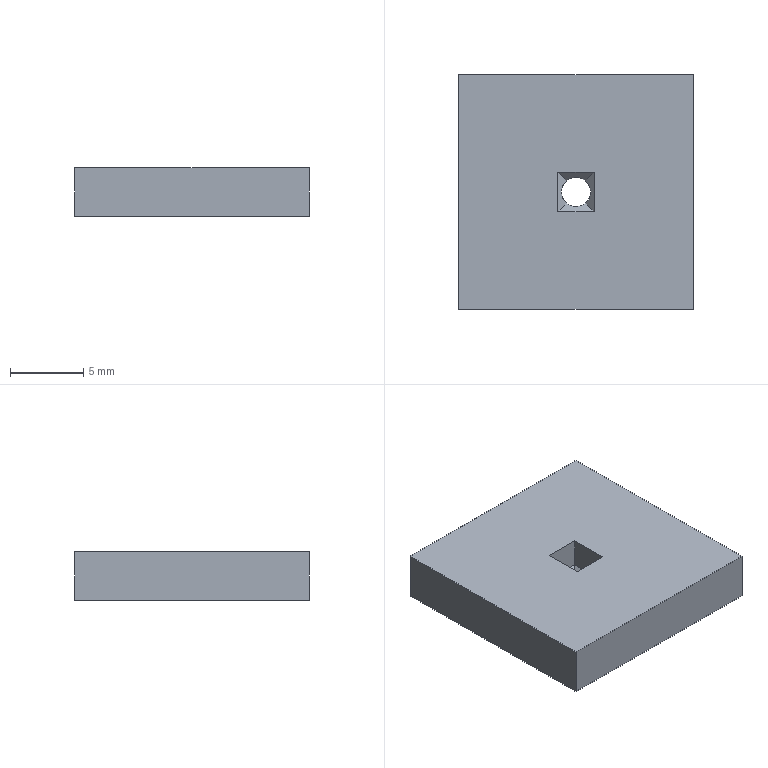Part | STEP file | 1 solid | 21 faces | box 16 x 16 x 3.3 mm | volume 788.101 mm3 | plane 19 | cylinder 2 | commonest cylinder face diameters 2 x2